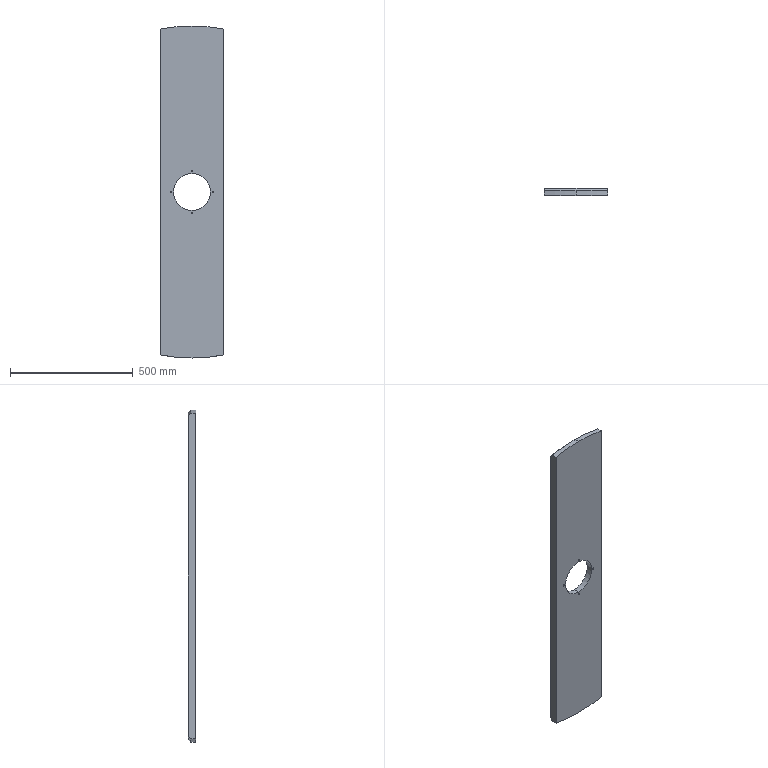Part | SolidWorks | features ICE 4, HoleWzd 2, Chamfer 1, Extrusion 1 | 1 solid | 23 faces | box 260 x 30 x 1350 mm | volume 9802887 mm3 | cylinder 15 | plane 5 | cone 3 | commonest cylinder face diameters 6.8 x8 1350 x3 150 x2 220 x2
STEP:
#1=CARTESIAN_POINT('',(0.,30.,-665.));
#2=VERTEX_POINT('',#1);
#3=CARTESIAN_POINT('',(-130.,30.,-652.169));
#4=VERTEX_POINT('',#3);
#5=CARTESIAN_POINT('',(0.,30.,0.));
#6=DIRECTION('',(0.,1.,0.));
#7=DIRECTION('',(0.,0.,1.));
#8=AXIS2_PLACEMENT_3D('',#5,#6,#7);
#9=CIRCLE('',#8,665.);
#10=EDGE_CURVE('',#2,#4,#9,.T.);
#11=ORIENTED_EDGE('',*,*,#10,.F.);
#12=CARTESIAN_POINT('',(0.,20.,-675.));
#13=VERTEX_POINT('',#12);
#14=CARTESIAN_POINT('',(0.,30.,-665.));
#15=DIRECTION('',(0.,-0.7071,-0.7071));
#16=VECTOR('',#15,1000.);
#17=LINE('',#14,#16);
#18=EDGE_CURVE('',#2,#13,#17,.T.);
#19=ORIENTED_EDGE('',*,*,#18,.T.);
#20=CARTESIAN_POINT('',(-130.,20.,-662.363));
#21=VERTEX_POINT('',#20);
#22=CARTESIAN_POINT('',(0.,20.,0.));
#23=DIRECTION('',(0.,-1.,0.));
#24=DIRECTION('',(0.,0.,1.));
#25=AXIS2_PLACEMENT_3D('',#22,#23,#24);
#26=CIRCLE('',#25,675.);
#27=EDGE_CURVE('',#21,#13,#26,.T.);
#28=ORIENTED_EDGE('',*,*,#27,.F.);
#29=CARTESIAN_POINT('',(-130.,30.,-652.169));
#30=CARTESIAN_POINT('',(-130.,26.667,-655.568));
#31=CARTESIAN_POINT('',(-130.,23.334,-658.966));
#32=CARTESIAN_POINT('',(-130.,20.,-662.363));
#33=B_SPLINE_CURVE_WITH_KNOTS('',3,(#29,#30,#31,#32),.UNSPECIFIED.,.F.,.F.,(4,4),(0.,0.01428),.UNSPECIFIED.);
#34=EDGE_CURVE('',#4,#21,#33,.T.);
#35=ORIENTED_EDGE('',*,*,#34,.F.);
#36=EDGE_LOOP('',(#11,#19,#28,#35));
#37=FACE_OUTER_BOUND('',#36,.T.);
#38=CARTESIAN_POINT('',(0.,30.,0.));
#39=DIRECTION('',(0.,-1.,0.));
#40=DIRECTION('',(0.,0.,-1.));
#41=AXIS2_PLACEMENT_3D('',#38,#39,#40);
#42=CONICAL_SURFACE('',#41,665.,0.7854);
#43=ADVANCED_FACE('',(#37),#42,.T.);
#44=CARTESIAN_POINT('',(-130.,0.,662.363));
#45=VERTEX_POINT('',#44);
#46=CARTESIAN_POINT('',(0.,0.,675.));
#47=VERTEX_POINT('',#46);
#48=CARTESIAN_POINT('',(0.,0.,0.));
#49=DIRECTION('',(0.,1.,0.));
#50=DIRECTION('',(0.,0.,1.));
#51=AXIS2_PLACEMENT_3D('',#48,#49,#50);
#52=CIRCLE('',#51,675.);
#53=EDGE_CURVE('',#45,#47,#52,.T.);
#54=ORIENTED_EDGE('',*,*,#53,.T.);
#55=CARTESIAN_POINT('',(0.,20.,675.));
#56=VERTEX_POINT('',#55);
#57=CARTESIAN_POINT('',(0.,0.,675.));
#58=DIRECTION('',(0.,1.,0.));
#59=VECTOR('',#58,1000.);
#60=LINE('',#57,#59);
#61=EDGE_CURVE('',#47,#56,#60,.T.);
#62=ORIENTED_EDGE('',*,*,#61,.T.);
#63=CARTESIAN_POINT('',(-130.,20.,662.363));
#64=VERTEX_POINT('',#63);
#65=CARTESIAN_POINT('',(0.,20.,0.));
#66=DIRECTION('',(0.,-1.,0.));
#67=DIRECTION('',(0.,0.,1.));
#68=AXIS2_PLACEMENT_3D('',#65,#66,#67);
#69=CIRCLE('',#68,675.);
#70=EDGE_CURVE('',#56,#64,#69,.T.);
#71=ORIENTED_EDGE('',*,*,#70,.T.);
#72=CARTESIAN_POINT('',(-130.,-0.001,662.363));
#73=DIRECTION('',(0.,1.,0.));
#74=VECTOR('',#73,1000.);
#75=LINE('',#72,#74);
#76=EDGE_CURVE('',#45,#64,#75,.T.);
#77=ORIENTED_EDGE('',*,*,#76,.F.);
#78=EDGE_LOOP('',(#54,#62,#71,#77));
#79=FACE_OUTER_BOUND('',#78,.T.);
#80=CARTESIAN_POINT('',(0.,0.,0.));
#81=DIRECTION('',(0.,1.,0.));
#82=DIRECTION('',(0.,0.,1.));
#83=AXIS2_PLACEMENT_3D('',#80,#81,#82);
#84=CYLINDRICAL_SURFACE('',#83,675.);
#85=ADVANCED_FACE('',(#79),#84,.T.);
#86=CARTESIAN_POINT('',(0.,0.,-88.4));
#87=VERTEX_POINT('',#86);
#88=CARTESIAN_POINT('',(0.,0.,-81.6));
#89=VERTEX_POINT('',#88);
#90=CARTESIAN_POINT('',(0.,0.,-85.));
#91=DIRECTION('',(0.,1.,0.));
#92=DIRECTION('',(0.,0.,1.));
#93=AXIS2_PLACEMENT_3D('',#90,#91,#92);
#94=CIRCLE('',#93,3.4);
#95=EDGE_CURVE('',#87,#89,#94,.T.);
#96=ORIENTED_EDGE('',*,*,#95,.F.);
#97=CARTESIAN_POINT('',(0.,25.,-88.4));
#98=VERTEX_POINT('',#97);
#99=CARTESIAN_POINT('',(0.,25.,-88.4));
#100=DIRECTION('',(0.,1.,0.));
#101=VECTOR('',#100,1000.);
#102=LINE('',#99,#101);
#103=EDGE_CURVE('',#87,#98,#102,.T.);
#104=ORIENTED_EDGE('',*,*,#103,.T.);
#105=CARTESIAN_POINT('',(0.,25.,-81.6));
#106=VERTEX_POINT('',#105);
#107=CARTESIAN_POINT('',(0.,25.,-85.));
#108=DIRECTION('',(0.,1.,0.));
#109=DIRECTION('',(0.,0.,1.));
#110=AXIS2_PLACEMENT_3D('',#107,#108,#109);
#111=CIRCLE('',#110,3.4);
#112=EDGE_CURVE('',#98,#106,#111,.T.);
#113=ORIENTED_EDGE('',*,*,#112,.T.);
#114=CARTESIAN_POINT('',(0.,25.,-81.6));
#115=DIRECTION('',(0.,1.,0.));
#116=VECTOR('',#115,1000.);
#117=LINE('',#114,#116);
#118=EDGE_CURVE('',#89,#106,#117,.T.);
#119=ORIENTED_EDGE('',*,*,#118,.F.);
#120=EDGE_LOOP('',(#96,#104,#113,#119));
#121=FACE_OUTER_BOUND('',#120,.T.);
#122=CARTESIAN_POINT('',(0.,25.,-85.));
#123=DIRECTION('',(0.,1.,0.));
#124=DIRECTION('',(0.,0.,1.));
#125=AXIS2_PLACEMENT_3D('',#122,#123,#124);
#126=CYLINDRICAL_SURFACE('',#125,3.4);
#127=ADVANCED_FACE('',(#121),#126,.F.);
#128=CARTESIAN_POINT('',(85.,0.,-3.4));
#129=VERTEX_POINT('',#128);
#130=CARTESIAN_POINT('',(85.,0.,3.4));
#131=VERTEX_POINT('',#130);
#132=CARTESIAN_POINT('',(85.,0.,0.));
#133=DIRECTION('',(0.,1.,0.));
#134=DIRECTION('',(0.,0.,1.));
#135=AXIS2_PLACEMENT_3D('',#132,#133,#134);
#136=CIRCLE('',#135,3.4);
#137=EDGE_CURVE('',#129,#131,#136,.T.);
#138=ORIENTED_EDGE('',*,*,#137,.F.);
#139=CARTESIAN_POINT('',(85.,25.,-3.4));
#140=VERTEX_POINT('',#139);
#141=CARTESIAN_POINT('',(85.,25.,-3.4));
#142=DIRECTION('',(0.,1.,0.));
#143=VECTOR('',#142,1000.);
#144=LINE('',#141,#143);
#145=EDGE_CURVE('',#129,#140,#144,.T.);
#146=ORIENTED_EDGE('',*,*,#145,.T.);
#147=CARTESIAN_POINT('',(85.,25.,3.4));
#148=VERTEX_POINT('',#147);
#149=CARTESIAN_POINT('',(85.,25.,0.));
#150=DIRECTION('',(0.,1.,0.));
#151=DIRECTION('',(0.,0.,1.));
#152=AXIS2_PLACEMENT_3D('',#149,#150,#151);
#153=CIRCLE('',#152,3.4);
#154=EDGE_CURVE('',#140,#148,#153,.T.);
#155=ORIENTED_EDGE('',*,*,#154,.T.);
#156=CARTESIAN_POINT('',(85.,25.,3.4));
#157=DIRECTION('',(0.,1.,0.));
#158=VECTOR('',#157,1000.);
#159=LINE('',#156,#158);
#160=EDGE_CURVE('',#131,#148,#159,.T.);
#161=ORIENTED_EDGE('',*,*,#160,.F.);
#162=EDGE_LOOP('',(#138,#146,#155,#161));
#163=FACE_OUTER_BOUND('',#162,.T.);
#164=CARTESIAN_POINT('',(85.,25.,0.));
#165=DIRECTION('',(0.,1.,0.));
#166=DIRECTION('',(0.,0.,1.));
#167=AXIS2_PLACEMENT_3D('',#164,#165,#166);
#168=CYLINDRICAL_SURFACE('',#167,3.4);
#169=ADVANCED_FACE('',(#163),#168,.F.);
#170=CARTESIAN_POINT('',(0.,0.,81.6));
#171=VERTEX_POINT('',#170);
#172=CARTESIAN_POINT('',(0.,0.,88.4));
#173=VERTEX_POINT('',#172);
#174=CARTESIAN_POINT('',(0.,0.,85.));
#175=DIRECTION('',(0.,1.,0.));
#176=DIRECTION('',(0.,0.,1.));
#177=AXIS2_PLACEMENT_3D('',#174,#175,#176);
#178=CIRCLE('',#177,3.4);
#179=EDGE_CURVE('',#171,#173,#178,.T.);
#180=ORIENTED_EDGE('',*,*,#179,.F.);
#181=CARTESIAN_POINT('',(0.,25.,81.6));
#182=VERTEX_POINT('',#181);
#183=CARTESIAN_POINT('',(0.,25.,81.6));
#184=DIRECTION('',(0.,1.,0.));
#185=VECTOR('',#184,1000.);
#186=LINE('',#183,#185);
#187=EDGE_CURVE('',#171,#182,#186,.T.);
#188=ORIENTED_EDGE('',*,*,#187,.T.);
#189=CARTESIAN_POINT('',(0.,25.,88.4));
#190=VERTEX_POINT('',#189);
#191=CARTESIAN_POINT('',(0.,25.,85.));
#192=DIRECTION('',(0.,1.,0.));
#193=DIRECTION('',(0.,0.,1.));
#194=AXIS2_PLACEMENT_3D('',#191,#192,#193);
#195=CIRCLE('',#194,3.4);
#196=EDGE_CURVE('',#182,#190,#195,.T.);
#197=ORIENTED_EDGE('',*,*,#196,.T.);
#198=CARTESIAN_POINT('',(0.,25.,88.4));
#199=DIRECTION('',(0.,1.,0.));
#200=VECTOR('',#199,1000.);
#201=LINE('',#198,#200);
#202=EDGE_CURVE('',#173,#190,#201,.T.);
#203=ORIENTED_EDGE('',*,*,#202,.F.);
#204=EDGE_LOOP('',(#180,#188,#197,#203));
#205=FACE_OUTER_BOUND('',#204,.T.);
#206=CARTESIAN_POINT('',(0.,25.,85.));
#207=DIRECTION('',(0.,1.,0.));
#208=DIRECTION('',(0.,0.,1.));
#209=AXIS2_PLACEMENT_3D('',#206,#207,#208);
#210=CYLINDRICAL_SURFACE('',#209,3.4);
#211=ADVANCED_FACE('',(#205),#210,.F.);
#212=CARTESIAN_POINT('',(-85.,0.,-3.4));
#213=VERTEX_POINT('',#212);
#214=CARTESIAN_POINT('',(-85.,0.,3.4));
#215=VERTEX_POINT('',#214);
#216=CARTESIAN_POINT('',(-85.,0.,0.));
#217=DIRECTION('',(0.,1.,0.));
#218=DIRECTION('',(0.,0.,1.));
#219=AXIS2_PLACEMENT_3D('',#216,#217,#218);
#220=CIRCLE('',#219,3.4);
#221=EDGE_CURVE('',#213,#215,#220,.T.);
#222=ORIENTED_EDGE('',*,*,#221,.F.);
#223=CARTESIAN_POINT('',(-85.,25.,-3.4));
#224=VERTEX_POINT('',#223);
#225=CARTESIAN_POINT('',(-85.,25.,-3.4));
#226=DIRECTION('',(0.,1.,0.));
#227=VECTOR('',#226,1000.);
#228=LINE('',#225,#227);
#229=EDGE_CURVE('',#213,#224,#228,.T.);
#230=ORIENTED_EDGE('',*,*,#229,.T.);
#231=CARTESIAN_POINT('',(-85.,25.,3.4));
#232=VERTEX_POINT('',#231);
#233=CARTESIAN_POINT('',(-85.,25.,0.));
#234=DIRECTION('',(0.,1.,0.));
#235=DIRECTION('',(0.,0.,1.));
#236=AXIS2_PLACEMENT_3D('',#233,#234,#235);
#237=CIRCLE('',#236,3.4);
#238=EDGE_CURVE('',#224,#232,#237,.T.);
#239=ORIENTED_EDGE('',*,*,#238,.T.);
#240=CARTESIAN_POINT('',(-85.,25.,3.4));
#241=DIRECTION('',(0.,1.,0.));
#242=VECTOR('',#241,1000.);
#243=LINE('',#240,#242);
#244=EDGE_CURVE('',#215,#232,#243,.T.);
#245=ORIENTED_EDGE('',*,*,#244,.F.);
#246=EDGE_LOOP('',(#222,#230,#239,#245));
#247=FACE_OUTER_BOUND('',#246,.T.);
#248=CARTESIAN_POINT('',(-85.,25.,0.));
#249=DIRECTION('',(0.,1.,0.));
#250=DIRECTION('',(0.,0.,1.));
#251=AXIS2_PLACEMENT_3D('',#248,#249,#250);
#252=CYLINDRICAL_SURFACE('',#251,3.4);
#253=ADVANCED_FACE('',(#247),#252,.F.);
#254=CARTESIAN_POINT('',(0.,25.,-110.));
#255=VERTEX_POINT('',#254);
#256=CARTESIAN_POINT('',(0.,25.,110.));
#257=VERTEX_POINT('',#256);
#258=CARTESIAN_POINT('',(0.,25.,0.));
#259=DIRECTION('',(0.,1.,0.));
#260=DIRECTION('',(0.,0.,1.));
#261=AXIS2_PLACEMENT_3D('',#258,#259,#260);
#262=CIRCLE('',#261,110.);
#263=EDGE_CURVE('',#255,#257,#262,.T.);
#264=ORIENTED_EDGE('',*,*,#263,.F.);
#265=CARTESIAN_POINT('',(0.,30.,-110.));
#266=VERTEX_POINT('',#265);
#267=CARTESIAN_POINT('',(0.,25.,-110.));
#268=DIRECTION('',(0.,1.,0.));
#269=VECTOR('',#268,1000.);
#270=LINE('',#267,#269);
#271=EDGE_CURVE('',#255,#266,#270,.T.);
#272=ORIENTED_EDGE('',*,*,#271,.T.);
#273=CARTESIAN_POINT('',(0.,30.,110.));
#274=VERTEX_POINT('',#273);
#275=CARTESIAN_POINT('',(0.,30.,0.));
#276=DIRECTION('',(0.,1.,0.));
#277=DIRECTION('',(0.,0.,1.));
#278=AXIS2_PLACEMENT_3D('',#275,#276,#277);
#279=CIRCLE('',#278,110.);
#280=EDGE_CURVE('',#266,#274,#279,.T.);
#281=ORIENTED_EDGE('',*,*,#280,.T.);
#282=CARTESIAN_POINT('',(0.,25.,110.));
#283=DIRECTION('',(0.,1.,0.));
#284=VECTOR('',#283,1000.);
#285=LINE('',#282,#284);
#286=EDGE_CURVE('',#257,#274,#285,.T.);
#287=ORIENTED_EDGE('',*,*,#286,.F.);
#288=EDGE_LOOP('',(#264,#272,#281,#287));
#289=FACE_OUTER_BOUND('',#288,.T.);
#290=CARTESIAN_POINT('',(0.,25.,0.));
#291=DIRECTION('',(0.,1.,0.));
#292=DIRECTION('',(0.,0.,1.));
#293=AXIS2_PLACEMENT_3D('',#290,#291,#292);
#294=CYLINDRICAL_SURFACE('',#293,110.);
#295=ADVANCED_FACE('',(#289),#294,.F.);
#296=CARTESIAN_POINT('',(0.,0.,75.));
#297=VERTEX_POINT('',#296);
#298=CARTESIAN_POINT('',(0.,0.,-75.));
#299=VERTEX_POINT('',#298);
#300=CARTESIAN_POINT('',(0.,0.,0.));
#301=DIRECTION('',(0.,-1.,0.));
#302=DIRECTION('',(0.,0.,1.));
#303=AXIS2_PLACEMENT_3D('',#300,#301,#302);
#304=CIRCLE('',#303,75.);
#305=EDGE_CURVE('',#297,#299,#304,.T.);
#306=ORIENTED_EDGE('',*,*,#305,.T.);
#307=CARTESIAN_POINT('',(0.,25.,-75.));
#308=VERTEX_POINT('',#307);
#309=CARTESIAN_POINT('',(0.,-0.001,-75.));
#310=DIRECTION('',(0.,1.,0.));
#311=VECTOR('',#310,1000.);
#312=LINE('',#309,#311);
#313=EDGE_CURVE('',#299,#308,#312,.T.);
#314=ORIENTED_EDGE('',*,*,#313,.T.);
#315=CARTESIAN_POINT('',(0.,25.,75.));
#316=VERTEX_POINT('',#315);
#317=CARTESIAN_POINT('',(0.,25.,0.));
#318=DIRECTION('',(0.,-1.,0.));
#319=DIRECTION('',(0.,0.,1.));
#320=AXIS2_PLACEMENT_3D('',#317,#318,#319);
#321=CIRCLE('',#320,75.);
#322=EDGE_CURVE('',#316,#308,#321,.T.);
#323=ORIENTED_EDGE('',*,*,#322,.F.);
#324=CARTESIAN_POINT('',(0.,-0.001,75.));
#325=DIRECTION('',(0.,1.,0.));
#326=VECTOR('',#325,1000.);
#327=LINE('',#324,#326);
#328=EDGE_CURVE('',#297,#316,#327,.T.);
#329=ORIENTED_EDGE('',*,*,#328,.F.);
#330=EDGE_LOOP('',(#306,#314,#323,#329));
#331=FACE_OUTER_BOUND('',#330,.T.);
#332=CARTESIAN_POINT('',(0.,-0.001,0.));
#333=DIRECTION('',(0.,1.,0.));
#334=DIRECTION('',(0.,0.,1.));
#335=AXIS2_PLACEMENT_3D('',#332,#333,#334);
#336=CYLINDRICAL_SURFACE('',#335,75.);
#337=ADVANCED_FACE('',(#331),#336,.F.);
#338=ORIENTED_EDGE('',*,*,#305,.F.);
#339=CARTESIAN_POINT('',(0.,0.,0.));
#340=DIRECTION('',(0.,-1.,0.));
#341=DIRECTION('',(0.,0.,1.));
#342=AXIS2_PLACEMENT_3D('',#339,#340,#341);
#343=CIRCLE('',#342,75.);
#344=EDGE_CURVE('',#299,#297,#343,.T.);
#345=ORIENTED_EDGE('',*,*,#344,.F.);
#346=EDGE_LOOP('',(#338,#345));
#347=FACE_BOUND('',#346,.T.);
#348=CARTESIAN_POINT('',(-85.,0.,0.));
#349=DIRECTION('',(0.,1.,0.));
#350=DIRECTION('',(0.,0.,1.));
#351=AXIS2_PLACEMENT_3D('',#348,#349,#350);
#352=CIRCLE('',#351,3.4);
#353=EDGE_CURVE('',#215,#213,#352,.T.);
#354=ORIENTED_EDGE('',*,*,#353,.T.);
#355=ORIENTED_EDGE('',*,*,#221,.T.);
#356=EDGE_LOOP('',(#354,#355));
#357=FACE_BOUND('',#356,.T.);
#358=CARTESIAN_POINT('',(0.,0.,85.));
#359=DIRECTION('',(0.,1.,0.));
#360=DIRECTION('',(0.,0.,1.));
#361=AXIS2_PLACEMENT_3D('',#358,#359,#360);
#362=CIRCLE('',#361,3.4);
#363=EDGE_CURVE('',#173,#171,#362,.T.);
#364=ORIENTED_EDGE('',*,*,#363,.T.);
#365=ORIENTED_EDGE('',*,*,#179,.T.);
#366=EDGE_LOOP('',(#364,#365));
#367=FACE_BOUND('',#366,.T.);
#368=CARTESIAN_POINT('',(85.,0.,0.));
#369=DIRECTION('',(0.,1.,0.));
#370=DIRECTION('',(0.,0.,1.));
#371=AXIS2_PLACEMENT_3D('',#368,#369,#370);
#372=CIRCLE('',#371,3.4);
#373=EDGE_CURVE('',#131,#129,#372,.T.);
#374=ORIENTED_EDGE('',*,*,#373,.T.);
#375=ORIENTED_EDGE('',*,*,#137,.T.);
#376=EDGE_LOOP('',(#374,#375));
#377=FACE_BOUND('',#376,.T.);
#378=CARTESIAN_POINT('',(0.,0.,-85.));
#379=DIRECTION('',(0.,1.,0.));
#380=DIRECTION('',(0.,0.,1.));
#381=AXIS2_PLACEMENT_3D('',#378,#379,#380);
#382=CIRCLE('',#381,3.4);
#383=EDGE_CURVE('',#89,#87,#382,.T.);
#384=ORIENTED_EDGE('',*,*,#383,.T.);
#385=ORIENTED_EDGE('',*,*,#95,.T.);
#386=EDGE_LOOP('',(#384,#385));
#387=FACE_BOUND('',#386,.T.);
#388=CARTESIAN_POINT('',(130.,0.,-662.363));
#389=VERTEX_POINT('',#388);
#390=CARTESIAN_POINT('',(-130.,0.,-662.363));
#391=VERTEX_POINT('',#390);
#392=CARTESIAN_POINT('',(0.,0.,0.));
#393=DIRECTION('',(0.,1.,0.));
#394=DIRECTION('',(0.,0.,1.));
#395=AXIS2_PLACEMENT_3D('',#392,#393,#394);
#396=CIRCLE('',#395,675.);
#397=EDGE_CURVE('',#389,#391,#396,.T.);
#398=ORIENTED_EDGE('',*,*,#397,.F.);
#399=CARTESIAN_POINT('',(130.,0.,662.363));
#400=VERTEX_POINT('',#399);
#401=CARTESIAN_POINT('',(130.,0.,0.));
#402=DIRECTION('',(0.,0.,1.));
#403=VECTOR('',#402,1000.);
#404=LINE('',#401,#403);
#405=EDGE_CURVE('',#389,#400,#404,.T.);
#406=ORIENTED_EDGE('',*,*,#405,.T.);
#407=CARTESIAN_POINT('',(0.,0.,0.));
#408=DIRECTION('',(0.,1.,0.));
#409=DIRECTION('',(0.,0.,1.));
#410=AXIS2_PLACEMENT_3D('',#407,#408,#409);
#411=CIRCLE('',#410,675.);
#412=EDGE_CURVE('',#47,#400,#411,.T.);
#413=ORIENTED_EDGE('',*,*,#412,.F.);
#414=ORIENTED_EDGE('',*,*,#53,.F.);
#415=CARTESIAN_POINT('',(-130.,0.,0.));
#416=DIRECTION('',(0.,0.,1.));
#417=VECTOR('',#416,1000.);
#418=LINE('',#415,#417);
#419=EDGE_CURVE('',#391,#45,#418,.T.);
#420=ORIENTED_EDGE('',*,*,#419,.F.);
#421=EDGE_LOOP('',(#398,#406,#413,#414,#420));
#422=FACE_OUTER_BOUND('',#421,.T.);
#423=CARTESIAN_POINT('',(0.,0.,0.));
#424=DIRECTION('',(0.,1.,0.));
#425=DIRECTION('',(0.,0.,1.));
#426=AXIS2_PLACEMENT_3D('',#423,#424,#425);
#427=PLANE('',#426);
#428=ADVANCED_FACE('',(#347,#357,#367,#377,#387,#422),#427,.F.);
#429=CARTESIAN_POINT('',(0.,30.,0.));
#430=DIRECTION('',(0.,1.,0.));
#431=DIRECTION('',(0.,0.,1.));
#432=AXIS2_PLACEMENT_3D('',#429,#430,#431);
#433=CIRCLE('',#432,110.);
#434=EDGE_CURVE('',#274,#266,#433,.T.);
#435=ORIENTED_EDGE('',*,*,#434,.F.);
#436=ORIENTED_EDGE('',*,*,#280,.F.);
#437=EDGE_LOOP('',(#435,#436));
#438=FACE_BOUND('',#437,.T.);
#439=CARTESIAN_POINT('',(-130.,30.,652.169));
#440=VERTEX_POINT('',#439);
#441=CARTESIAN_POINT('',(-130.,30.,0.));
#442=DIRECTION('',(0.,0.,-1.));
#443=VECTOR('',#442,1000.);
#444=LINE('',#441,#443);
#445=EDGE_CURVE('',#440,#4,#444,.T.);
#446=ORIENTED_EDGE('',*,*,#445,.F.);
#447=CARTESIAN_POINT('',(130.,30.,652.169));
#448=VERTEX_POINT('',#447);
#449=CARTESIAN_POINT('',(0.,30.,0.));
#450=DIRECTION('',(0.,1.,0.));
#451=DIRECTION('',(0.,0.,1.));
#452=AXIS2_PLACEMENT_3D('',#449,#450,#451);
#453=CIRCLE('',#452,665.);
#454=EDGE_CURVE('',#440,#448,#453,.T.);
#455=ORIENTED_EDGE('',*,*,#454,.T.);
#456=CARTESIAN_POINT('',(130.,30.,-652.169));
#457=VERTEX_POINT('',#456);
#458=CARTESIAN_POINT('',(130.,30.,0.));
#459=DIRECTION('',(0.,0.,-1.));
#460=VECTOR('',#459,1000.);
#461=LINE('',#458,#460);
#462=EDGE_CURVE('',#448,#457,#461,.T.);
#463=ORIENTED_EDGE('',*,*,#462,.T.);
#464=CARTESIAN_POINT('',(0.,30.,0.));
#465=DIRECTION('',(0.,1.,0.));
#466=DIRECTION('',(0.,0.,1.));
#467=AXIS2_PLACEMENT_3D('',#464,#465,#466);
#468=CIRCLE('',#467,665.);
#469=EDGE_CURVE('',#457,#2,#468,.T.);
#470=ORIENTED_EDGE('',*,*,#469,.T.);
#471=ORIENTED_EDGE('',*,*,#10,.T.);
#472=EDGE_LOOP('',(#446,#455,#463,#470,#471));
#473=FACE_OUTER_BOUND('',#472,.T.);
#474=CARTESIAN_POINT('',(0.,30.,0.));
#475=DIRECTION('',(0.,1.,0.));
#476=DIRECTION('',(0.,0.,1.));
#477=AXIS2_PLACEMENT_3D('',#474,#475,#476);
#478=PLANE('',#477);
#479=ADVANCED_FACE('',(#438,#473),#478,.T.);
#480=ORIENTED_EDGE('',*,*,#313,.F.);
#481=ORIENTED_EDGE('',*,*,#344,.T.);
#482=ORIENTED_EDGE('',*,*,#328,.T.);
#483=CARTESIAN_POINT('',(0.,25.,0.));
#484=DIRECTION('',(0.,-1.,0.));
#485=DIRECTION('',(0.,0.,1.));
#486=AXIS2_PLACEMENT_3D('',#483,#484,#485);
#487=CIRCLE('',#486,75.);
#488=EDGE_CURVE('',#308,#316,#487,.T.);
#489=ORIENTED_EDGE('',*,*,#488,.F.);
#490=EDGE_LOOP('',(#480,#481,#482,#489));
#491=FACE_OUTER_BOUND('',#490,.T.);
#492=CARTESIAN_POINT('',(0.,-0.001,0.));
#493=DIRECTION('',(0.,1.,0.));
#494=DIRECTION('',(0.,0.,1.));
#495=AXIS2_PLACEMENT_3D('',#492,#493,#494);
#496=CYLINDRICAL_SURFACE('',#495,75.);
#497=ADVANCED_FACE('',(#491),#496,.F.);
#498=ORIENTED_EDGE('',*,*,#76,.T.);
#499=CARTESIAN_POINT('',(-130.,20.,662.363));
#500=CARTESIAN_POINT('',(-130.,23.334,658.966));
#501=CARTESIAN_POINT('',(-130.,26.667,655.568));
#502=CARTESIAN_POINT('',(-130.,30.,652.169));
#503=B_SPLINE_CURVE_WITH_KNOTS('',3,(#499,#500,#501,#502),.UNSPECIFIED.,.F.,.F.,(4,4),(0.,0.01428),.UNSPECIFIED.);
#504=EDGE_CURVE('',#64,#440,#503,.T.);
#505=ORIENTED_EDGE('',*,*,#504,.T.);
#506=ORIENTED_EDGE('',*,*,#445,.T.);
#507=ORIENTED_EDGE('',*,*,#34,.T.);
#508=CARTESIAN_POINT('',(-130.,-0.001,-662.363));
#509=DIRECTION('',(0.,1.,0.));
#510=VECTOR('',#509,1000.);
#511=LINE('',#508,#510);
#512=EDGE_CURVE('',#391,#21,#511,.T.);
#513=ORIENTED_EDGE('',*,*,#512,.F.);
#514=ORIENTED_EDGE('',*,*,#419,.T.);
#515=EDGE_LOOP('',(#498,#505,#506,#507,#513,#514));
#516=FACE_OUTER_BOUND('',#515,.T.);
#517=CARTESIAN_POINT('',(-130.,-0.001,0.));
#518=DIRECTION('',(1.,0.,0.));
#519=DIRECTION('',(0.,0.,-1.));
#520=AXIS2_PLACEMENT_3D('',#517,#518,#519);
#521=PLANE('',#520);
#522=ADVANCED_FACE('',(#516),#521,.F.);
#523=ORIENTED_EDGE('',*,*,#462,.F.);
#524=CARTESIAN_POINT('',(130.,20.,662.363));
#525=VERTEX_POINT('',#524);
#526=CARTESIAN_POINT('',(130.,30.,652.169));
#527=CARTESIAN_POINT('',(130.,26.667,655.568));
#528=CARTESIAN_POINT('',(130.,23.334,658.966));
#529=CARTESIAN_POINT('',(130.,20.,662.363));
#530=B_SPLINE_CURVE_WITH_KNOTS('',3,(#526,#527,#528,#529),.UNSPECIFIED.,.F.,.F.,(4,4),(0.,0.01428),.UNSPECIFIED.);
#531=EDGE_CURVE('',#448,#525,#530,.T.);
#532=ORIENTED_EDGE('',*,*,#531,.T.);
#533=CARTESIAN_POINT('',(130.,-0.001,662.363));
#534=DIRECTION('',(0.,1.,0.));
#535=VECTOR('',#534,1000.);
#536=LINE('',#533,#535);
#537=EDGE_CURVE('',#400,#525,#536,.T.);
#538=ORIENTED_EDGE('',*,*,#537,.F.);
#539=ORIENTED_EDGE('',*,*,#405,.F.);
#540=CARTESIAN_POINT('',(130.,20.,-662.363));
#541=VERTEX_POINT('',#540);
#542=CARTESIAN_POINT('',(130.,-0.001,-662.363));
#543=DIRECTION('',(0.,1.,0.));
#544=VECTOR('',#543,1000.);
#545=LINE('',#542,#544);
#546=EDGE_CURVE('',#389,#541,#545,.T.);
#547=ORIENTED_EDGE('',*,*,#546,.T.);
#548=CARTESIAN_POINT('',(130.,20.,-662.363));
#549=CARTESIAN_POINT('',(130.,23.334,-658.966));
#550=CARTESIAN_POINT('',(130.,26.667,-655.568));
#551=CARTESIAN_POINT('',(130.,30.,-652.169));
#552=B_SPLINE_CURVE_WITH_KNOTS('',3,(#548,#549,#550,#551),.UNSPECIFIED.,.F.,.F.,(4,4),(0.,0.01428),.UNSPECIFIED.);
#553=EDGE_CURVE('',#541,#457,#552,.T.);
#554=ORIENTED_EDGE('',*,*,#553,.T.);
#555=EDGE_LOOP('',(#523,#532,#538,#539,#547,#554));
#556=FACE_OUTER_BOUND('',#555,.T.);
#557=CARTESIAN_POINT('',(130.,-0.001,0.));
#558=DIRECTION('',(1.,0.,0.));
#559=DIRECTION('',(0.,0.,-1.));
#560=AXIS2_PLACEMENT_3D('',#557,#558,#559);
#561=PLANE('',#560);
#562=ADVANCED_FACE('',(#556),#561,.T.);
#563=CARTESIAN_POINT('',(0.,25.,-85.));
#564=DIRECTION('',(0.,1.,0.));
#565=DIRECTION('',(0.,0.,1.));
#566=AXIS2_PLACEMENT_3D('',#563,#564,#565);
#567=CIRCLE('',#566,3.4);
#568=EDGE_CURVE('',#106,#98,#567,.T.);
#569=ORIENTED_EDGE('',*,*,#568,.F.);
#570=ORIENTED_EDGE('',*,*,#112,.F.);
#571=EDGE_LOOP('',(#569,#570));
#572=FACE_BOUND('',#571,.T.);
#573=CARTESIAN_POINT('',(85.,25.,0.));
#574=DIRECTION('',(0.,1.,0.));
#575=DIRECTION('',(0.,0.,1.));
#576=AXIS2_PLACEMENT_3D('',#573,#574,#575);
#577=CIRCLE('',#576,3.4);
#578=EDGE_CURVE('',#148,#140,#577,.T.);
#579=ORIENTED_EDGE('',*,*,#578,.F.);
#580=ORIENTED_EDGE('',*,*,#154,.F.);
#581=EDGE_LOOP('',(#579,#580));
#582=FACE_BOUND('',#581,.T.);
#583=CARTESIAN_POINT('',(0.,25.,85.));
#584=DIRECTION('',(0.,1.,0.));
#585=DIRECTION('',(0.,0.,1.));
#586=AXIS2_PLACEMENT_3D('',#583,#584,#585);
#587=CIRCLE('',#586,3.4);
#588=EDGE_CURVE('',#190,#182,#587,.T.);
#589=ORIENTED_EDGE('',*,*,#588,.F.);
#590=ORIENTED_EDGE('',*,*,#196,.F.);
#591=EDGE_LOOP('',(#589,#590));
#592=FACE_BOUND('',#591,.T.);
#593=CARTESIAN_POINT('',(-85.,25.,0.));
#594=DIRECTION('',(0.,1.,0.));
#595=DIRECTION('',(0.,0.,1.));
#596=AXIS2_PLACEMENT_3D('',#593,#594,#595);
#597=CIRCLE('',#596,3.4);
#598=EDGE_CURVE('',#232,#224,#597,.T.);
#599=ORIENTED_EDGE('',*,*,#598,.F.);
#600=ORIENTED_EDGE('',*,*,#238,.F.);
#601=EDGE_LOOP('',(#599,#600));
#602=FACE_BOUND('',#601,.T.);
#603=CARTESIAN_POINT('',(0.,25.,0.));
#604=DIRECTION('',(0.,1.,0.));
#605=DIRECTION('',(0.,0.,1.));
#606=AXIS2_PLACEMENT_3D('',#603,#604,#605);
#607=CIRCLE('',#606,110.);
#608=EDGE_CURVE('',#257,#255,#607,.T.);
#609=ORIENTED_EDGE('',*,*,#608,.T.);
#610=ORIENTED_EDGE('',*,*,#263,.T.);
#611=EDGE_LOOP('',(#609,#610));
#612=FACE_OUTER_BOUND('',#611,.T.);
#613=ORIENTED_EDGE('',*,*,#322,.T.);
#614=ORIENTED_EDGE('',*,*,#488,.T.);
#615=EDGE_LOOP('',(#613,#614));
#616=FACE_BOUND('',#615,.T.);
#617=CARTESIAN_POINT('',(0.,25.,0.));
#618=DIRECTION('',(0.,1.,0.));
#619=DIRECTION('',(0.,0.,1.));
#620=AXIS2_PLACEMENT_3D('',#617,#618,#619);
#621=PLANE('',#620);
#622=ADVANCED_FACE('',(#572,#582,#592,#602,#612,#616),#621,.T.);
#623=ORIENTED_EDGE('',*,*,#271,.F.);
#624=ORIENTED_EDGE('',*,*,#608,.F.);
#625=ORIENTED_EDGE('',*,*,#286,.T.);
#626=ORIENTED_EDGE('',*,*,#434,.T.);
#627=EDGE_LOOP('',(#623,#624,#625,#626));
#628=FACE_OUTER_BOUND('',#627,.T.);
#629=CARTESIAN_POINT('',(0.,25.,0.));
#630=DIRECTION('',(0.,1.,0.));
#631=DIRECTION('',(0.,0.,1.));
#632=AXIS2_PLACEMENT_3D('',#629,#630,#631);
#633=CYLINDRICAL_SURFACE('',#632,110.);
#634=ADVANCED_FACE('',(#628),#633,.F.);
#635=ORIENTED_EDGE('',*,*,#229,.F.);
#636=ORIENTED_EDGE('',*,*,#353,.F.);
#637=ORIENTED_EDGE('',*,*,#244,.T.);
#638=ORIENTED_EDGE('',*,*,#598,.T.);
#639=EDGE_LOOP('',(#635,#636,#637,#638));
#640=FACE_OUTER_BOUND('',#639,.T.);
#641=CARTESIAN_POINT('',(-85.,25.,0.));
#642=DIRECTION('',(0.,1.,0.));
#643=DIRECTION('',(0.,0.,1.));
#644=AXIS2_PLACEMENT_3D('',#641,#642,#643);
#645=CYLINDRICAL_SURFACE('',#644,3.4);
#646=ADVANCED_FACE('',(#640),#645,.F.);
#647=ORIENTED_EDGE('',*,*,#187,.F.);
#648=ORIENTED_EDGE('',*,*,#363,.F.);
#649=ORIENTED_EDGE('',*,*,#202,.T.);
#650=ORIENTED_EDGE('',*,*,#588,.T.);
#651=EDGE_LOOP('',(#647,#648,#649,#650));
#652=FACE_OUTER_BOUND('',#651,.T.);
#653=CARTESIAN_POINT('',(0.,25.,85.));
#654=DIRECTION('',(0.,1.,0.));
#655=DIRECTION('',(0.,0.,1.));
#656=AXIS2_PLACEMENT_3D('',#653,#654,#655);
#657=CYLINDRICAL_SURFACE('',#656,3.4);
#658=ADVANCED_FACE('',(#652),#657,.F.);
#659=ORIENTED_EDGE('',*,*,#145,.F.);
#660=ORIENTED_EDGE('',*,*,#373,.F.);
#661=ORIENTED_EDGE('',*,*,#160,.T.);
#662=ORIENTED_EDGE('',*,*,#578,.T.);
#663=EDGE_LOOP('',(#659,#660,#661,#662));
#664=FACE_OUTER_BOUND('',#663,.T.);
#665=CARTESIAN_POINT('',(85.,25.,0.));
#666=DIRECTION('',(0.,1.,0.));
#667=DIRECTION('',(0.,0.,1.));
#668=AXIS2_PLACEMENT_3D('',#665,#666,#667);
#669=CYLINDRICAL_SURFACE('',#668,3.4);
#670=ADVANCED_FACE('',(#664),#669,.F.);
#671=ORIENTED_EDGE('',*,*,#103,.F.);
#672=ORIENTED_EDGE('',*,*,#383,.F.);
#673=ORIENTED_EDGE('',*,*,#118,.T.);
#674=ORIENTED_EDGE('',*,*,#568,.T.);
#675=EDGE_LOOP('',(#671,#672,#673,#674));
#676=FACE_OUTER_BOUND('',#675,.T.);
#677=CARTESIAN_POINT('',(0.,25.,-85.));
#678=DIRECTION('',(0.,1.,0.));
#679=DIRECTION('',(0.,0.,1.));
#680=AXIS2_PLACEMENT_3D('',#677,#678,#679);
#681=CYLINDRICAL_SURFACE('',#680,3.4);
#682=ADVANCED_FACE('',(#676),#681,.F.);
#683=ORIENTED_EDGE('',*,*,#61,.F.);
#684=ORIENTED_EDGE('',*,*,#412,.T.);
#685=ORIENTED_EDGE('',*,*,#537,.T.);
#686=CARTESIAN_POINT('',(0.,20.,0.));
#687=DIRECTION('',(0.,-1.,0.));
#688=DIRECTION('',(0.,0.,1.));
#689=AXIS2_PLACEMENT_3D('',#686,#687,#688);
#690=CIRCLE('',#689,675.);
#691=EDGE_CURVE('',#525,#56,#690,.T.);
#692=ORIENTED_EDGE('',*,*,#691,.T.);
#693=EDGE_LOOP('',(#683,#684,#685,#692));
#694=FACE_OUTER_BOUND('',#693,.T.);
#695=CARTESIAN_POINT('',(0.,0.,0.));
#696=DIRECTION('',(0.,1.,0.));
#697=DIRECTION('',(0.,0.,1.));
#698=AXIS2_PLACEMENT_3D('',#695,#696,#697);
#699=CYLINDRICAL_SURFACE('',#698,675.);
#700=ADVANCED_FACE('',(#694),#699,.T.);
#701=ORIENTED_EDGE('',*,*,#512,.T.);
#702=ORIENTED_EDGE('',*,*,#27,.T.);
#703=CARTESIAN_POINT('',(0.,20.,0.));
#704=DIRECTION('',(0.,-1.,0.));
#705=DIRECTION('',(0.,0.,1.));
#706=AXIS2_PLACEMENT_3D('',#703,#704,#705);
#707=CIRCLE('',#706,675.);
#708=EDGE_CURVE('',#13,#541,#707,.T.);
#709=ORIENTED_EDGE('',*,*,#708,.T.);
#710=ORIENTED_EDGE('',*,*,#546,.F.);
#711=ORIENTED_EDGE('',*,*,#397,.T.);
#712=EDGE_LOOP('',(#701,#702,#709,#710,#711));
#713=FACE_OUTER_BOUND('',#712,.T.);
#714=CARTESIAN_POINT('',(0.,0.,0.));
#715=DIRECTION('',(0.,1.,0.));
#716=DIRECTION('',(0.,0.,1.));
#717=AXIS2_PLACEMENT_3D('',#714,#715,#716);
#718=CYLINDRICAL_SURFACE('',#717,675.);
#719=ADVANCED_FACE('',(#713),#718,.T.);
#720=ORIENTED_EDGE('',*,*,#504,.F.);
#721=ORIENTED_EDGE('',*,*,#70,.F.);
#722=ORIENTED_EDGE('',*,*,#691,.F.);
#723=ORIENTED_EDGE('',*,*,#531,.F.);
#724=ORIENTED_EDGE('',*,*,#454,.F.);
#725=EDGE_LOOP('',(#720,#721,#722,#723,#724));
#726=FACE_OUTER_BOUND('',#725,.T.);
#727=CARTESIAN_POINT('',(0.,30.,0.));
#728=DIRECTION('',(0.,-1.,0.));
#729=DIRECTION('',(0.,0.,-1.));
#730=AXIS2_PLACEMENT_3D('',#727,#728,#729);
#731=CONICAL_SURFACE('',#730,665.,0.7854);
#732=ADVANCED_FACE('',(#726),#731,.T.);
#733=ORIENTED_EDGE('',*,*,#18,.F.);
#734=ORIENTED_EDGE('',*,*,#469,.F.);
#735=ORIENTED_EDGE('',*,*,#553,.F.);
#736=ORIENTED_EDGE('',*,*,#708,.F.);
#737=EDGE_LOOP('',(#733,#734,#735,#736));
#738=FACE_OUTER_BOUND('',#737,.T.);
#739=CARTESIAN_POINT('',(0.,30.,0.));
#740=DIRECTION('',(0.,-1.,0.));
#741=DIRECTION('',(0.,0.,-1.));
#742=AXIS2_PLACEMENT_3D('',#739,#740,#741);
#743=CONICAL_SURFACE('',#742,665.,0.7854);
#744=ADVANCED_FACE('',(#738),#743,.T.);
#745=CLOSED_SHELL('',(#43,#85,#127,#169,#211,#253,#295,#337,#428,#479,#497,#522,#562,#622,#634,#646,#658,#670,#682,#700,#719,#732,#744));
#746=MANIFOLD_SOLID_BREP('',#745);
#747=CARTESIAN_POINT('',(0.,0.,0.));
#748=DIRECTION('',(0.,0.,1.));
#749=DIRECTION('',(1.,0.,0.));
#750=AXIS2_PLACEMENT_3D('',#747,#748,#749);
#751=(LENGTH_UNIT()NAMED_UNIT(*)SI_UNIT(.MILLI.,.METRE.));
#752=UNCERTAINTY_MEASURE_WITH_UNIT(LENGTH_MEASURE(0.00001),#751,'','');
#753=(NAMED_UNIT(*)PLANE_ANGLE_UNIT()SI_UNIT($,.RADIAN.));
#754=(NAMED_UNIT(*)SI_UNIT($,.STERADIAN.)SOLID_ANGLE_UNIT());
#755=(GEOMETRIC_REPRESENTATION_CONTEXT(3)GLOBAL_UNCERTAINTY_ASSIGNED_CONTEXT((#752))GLOBAL_UNIT_ASSIGNED_CONTEXT((#751,#753,#754))REPRESENTATION_CONTEXT('',''));
#756=ADVANCED_BREP_SHAPE_REPRESENTATION('',(#746,#750),#755);